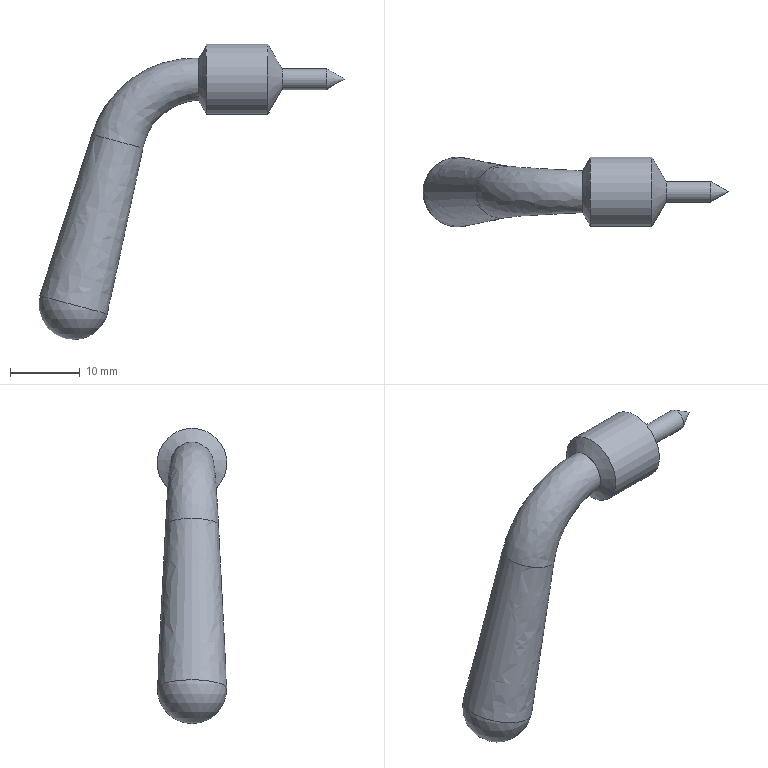Part | NX | features SKETCH 4, DATUM_CSYS 3, DATUM_ON_PATH 2, SKIN 1, SPHERE 1, SWP104 1 | 3 solids | 11 faces | box 43.874 x 10 x 42.344 mm | volume 3412 mm3 | cone 3 | plane 3 | cylinder 2 | spline 2 | sphere 1 | commonest cylinder face diameters 3 x1 10 x1
STEP:
#1=CARTESIAN_POINT('',(18.402,0.,-1.5));
#2=VERTEX_POINT('',#1);
#3=CARTESIAN_POINT('',(18.402,0.,0.));
#4=DIRECTION('',(1.,0.,0.));
#5=DIRECTION('',(0.,0.,-1.));
#6=AXIS2_PLACEMENT_3D('',#3,#4,#5);
#7=CIRCLE('',#6,1.5);
#8=EDGE_CURVE('',#2,#2,#7,.T.);
#9=ORIENTED_EDGE('',*,*,#8,.T.);
#10=EDGE_LOOP('',(#9));
#11=FACE_BOUND('',#10,.T.);
#12=CARTESIAN_POINT('',(21.,0.,0.));
#13=VERTEX_POINT('',#12);
#14=VERTEX_LOOP('',#13);
#15=FACE_BOUND('',#14,.T.);
#16=CARTESIAN_POINT('',(21.,0.,0.));
#17=DIRECTION('',(-1.,0.,0.));
#18=DIRECTION('',(0.,0.,1.));
#19=AXIS2_PLACEMENT_3D('',#16,#17,#18);
#20=CONICAL_SURFACE('',#19,0.,0.5236);
#21=ADVANCED_FACE('',(#11,#15),#20,.T.);
#22=CARTESIAN_POINT('',(12.,0.,-1.5));
#23=VERTEX_POINT('',#22);
#24=CARTESIAN_POINT('',(12.,0.,0.));
#25=DIRECTION('',(1.,0.,0.));
#26=DIRECTION('',(0.,0.,-1.));
#27=AXIS2_PLACEMENT_3D('',#24,#25,#26);
#28=CIRCLE('',#27,1.5);
#29=EDGE_CURVE('',#23,#23,#28,.T.);
#30=ORIENTED_EDGE('',*,*,#29,.T.);
#31=EDGE_LOOP('',(#30));
#32=FACE_BOUND('',#31,.T.);
#33=ORIENTED_EDGE('',*,*,#8,.F.);
#34=EDGE_LOOP('',(#33));
#35=FACE_BOUND('',#34,.T.);
#36=CARTESIAN_POINT('',(0.,0.,0.));
#37=DIRECTION('',(1.,0.,0.));
#38=DIRECTION('',(0.,0.,-1.));
#39=AXIS2_PLACEMENT_3D('',#36,#37,#38);
#40=CYLINDRICAL_SURFACE('',#39,1.5);
#41=ADVANCED_FACE('',(#32,#35),#40,.T.);
#42=CARTESIAN_POINT('',(9.979,0.,-5.));
#43=VERTEX_POINT('',#42);
#44=CARTESIAN_POINT('',(9.979,0.,0.));
#45=DIRECTION('',(1.,0.,0.));
#46=DIRECTION('',(0.,0.,-1.));
#47=AXIS2_PLACEMENT_3D('',#44,#45,#46);
#48=CIRCLE('',#47,5.);
#49=EDGE_CURVE('',#43,#43,#48,.T.);
#50=ORIENTED_EDGE('',*,*,#49,.T.);
#51=EDGE_LOOP('',(#50));
#52=FACE_BOUND('',#51,.T.);
#53=ORIENTED_EDGE('',*,*,#29,.F.);
#54=EDGE_LOOP('',(#53));
#55=FACE_BOUND('',#54,.T.);
#56=CARTESIAN_POINT('',(12.,0.,0.));
#57=DIRECTION('',(-1.,0.,0.));
#58=DIRECTION('',(0.,0.,1.));
#59=AXIS2_PLACEMENT_3D('',#56,#57,#58);
#60=CONICAL_SURFACE('',#59,1.5,1.047);
#61=ADVANCED_FACE('',(#52,#55),#60,.T.);
#62=CARTESIAN_POINT('',(1.155,0.,-5.));
#63=VERTEX_POINT('',#62);
#64=CARTESIAN_POINT('',(1.155,0.,0.));
#65=DIRECTION('',(1.,0.,0.));
#66=DIRECTION('',(0.,0.,-1.));
#67=AXIS2_PLACEMENT_3D('',#64,#65,#66);
#68=CIRCLE('',#67,5.);
#69=EDGE_CURVE('',#63,#63,#68,.T.);
#70=ORIENTED_EDGE('',*,*,#69,.T.);
#71=EDGE_LOOP('',(#70));
#72=FACE_BOUND('',#71,.T.);
#73=ORIENTED_EDGE('',*,*,#49,.F.);
#74=EDGE_LOOP('',(#73));
#75=FACE_BOUND('',#74,.T.);
#76=CARTESIAN_POINT('',(0.,0.,0.));
#77=DIRECTION('',(1.,0.,0.));
#78=DIRECTION('',(0.,0.,-1.));
#79=AXIS2_PLACEMENT_3D('',#76,#77,#78);
#80=CYLINDRICAL_SURFACE('',#79,5.);
#81=ADVANCED_FACE('',(#72,#75),#80,.T.);
#82=CARTESIAN_POINT('',(0.,0.,-3.));
#83=VERTEX_POINT('',#82);
#84=CARTESIAN_POINT('',(0.,0.,0.));
#85=DIRECTION('',(1.,0.,0.));
#86=DIRECTION('',(0.,0.,-1.));
#87=AXIS2_PLACEMENT_3D('',#84,#85,#86);
#88=CIRCLE('',#87,3.);
#89=EDGE_CURVE('',#83,#83,#88,.T.);
#90=ORIENTED_EDGE('',*,*,#89,.T.);
#91=EDGE_LOOP('',(#90));
#92=FACE_BOUND('',#91,.T.);
#93=ORIENTED_EDGE('',*,*,#69,.F.);
#94=EDGE_LOOP('',(#93));
#95=FACE_BOUND('',#94,.T.);
#96=CARTESIAN_POINT('',(1.155,0.,0.));
#97=DIRECTION('',(1.,0.,0.));
#98=DIRECTION('',(0.,0.,-1.));
#99=AXIS2_PLACEMENT_3D('',#96,#97,#98);
#100=CONICAL_SURFACE('',#99,5.,1.047);
#101=ADVANCED_FACE('',(#92,#95),#100,.T.);
#102=ORIENTED_EDGE('',*,*,#89,.F.);
#103=EDGE_LOOP('',(#102));
#104=FACE_BOUND('',#103,.T.);
#105=CARTESIAN_POINT('',(0.,3.,0.));
#106=DIRECTION('',(-1.,0.,0.));
#107=DIRECTION('',(0.,0.,1.));
#108=AXIS2_PLACEMENT_3D('',#105,#106,#107);
#109=PLANE('',#108);
#110=ADVANCED_FACE('',(#104),#109,.T.);
#111=CLOSED_SHELL('',(#21,#41,#61,#81,#101,#110));
#112=MANIFOLD_SOLID_BREP('',#111);
#113=CARTESIAN_POINT('',(-17.874,0.,-37.344));
#114=VERTEX_POINT('',#113);
#115=VERTEX_LOOP('',#114);
#116=FACE_BOUND('',#115,.T.);
#117=CARTESIAN_POINT('',(-17.874,0.,-32.344));
#118=DIRECTION('',(0.,0.,1.));
#119=DIRECTION('',(1.,0.,0.));
#120=AXIS2_PLACEMENT_3D('',#117,#118,#119);
#121=SPHERICAL_SURFACE('',#120,5.);
#122=ADVANCED_FACE('',(#116),#121,.T.);
#123=CLOSED_SHELL('',(#122));
#124=MANIFOLD_SOLID_BREP('',#123);
#125=CARTESIAN_POINT('',(-22.704,0.,-31.05));
#126=VERTEX_POINT('',#125);
#127=CARTESIAN_POINT('',(-22.649,-0.9378,-31.064));
#128=CARTESIAN_POINT('',(-22.729,-0.03039,-31.043));
#129=CARTESIAN_POINT('',(-22.657,0.8728,-31.062));
#130=CARTESIAN_POINT('',(-22.415,1.799,-31.127));
#131=CARTESIAN_POINT('',(-21.975,2.707,-31.245));
#132=CARTESIAN_POINT('',(-21.352,3.522,-31.412));
#133=CARTESIAN_POINT('',(-20.577,4.186,-31.619));
#134=CARTESIAN_POINT('',(-19.707,4.662,-31.853));
#135=CARTESIAN_POINT('',(-18.796,4.938,-32.097));
#136=CARTESIAN_POINT('',(-17.921,5.026,-32.331));
#137=CARTESIAN_POINT('',(-17.048,4.956,-32.565));
#138=CARTESIAN_POINT('',(-16.137,4.701,-32.809));
#139=CARTESIAN_POINT('',(-15.26,4.246,-33.044));
#140=CARTESIAN_POINT('',(-14.472,3.6,-33.255));
#141=CARTESIAN_POINT('',(-13.831,2.798,-33.427));
#142=CARTESIAN_POINT('',(-13.371,1.897,-33.55));
#143=CARTESIAN_POINT('',(-13.104,0.954,-33.622));
#144=CARTESIAN_POINT('',(-13.02,0.04792,-33.645));
#145=CARTESIAN_POINT('',(-13.087,-0.8557,-33.626));
#146=CARTESIAN_POINT('',(-13.334,-1.798,-33.56));
#147=CARTESIAN_POINT('',(-13.773,-2.707,-33.443));
#148=CARTESIAN_POINT('',(-14.397,-3.522,-33.275));
#149=CARTESIAN_POINT('',(-15.172,-4.186,-33.068));
#150=CARTESIAN_POINT('',(-16.042,-4.662,-32.835));
#151=CARTESIAN_POINT('',(-16.953,-4.938,-32.591));
#152=CARTESIAN_POINT('',(-17.828,-5.026,-32.356));
#153=CARTESIAN_POINT('',(-18.701,-4.956,-32.122));
#154=CARTESIAN_POINT('',(-19.612,-4.701,-31.878));
#155=CARTESIAN_POINT('',(-20.489,-4.246,-31.643));
#156=CARTESIAN_POINT('',(-21.276,-3.6,-31.432));
#157=CARTESIAN_POINT('',(-21.918,-2.798,-31.26));
#158=CARTESIAN_POINT('',(-22.378,-1.897,-31.137));
#159=CARTESIAN_POINT('',(-22.649,-0.9378,-31.064));
#160=CARTESIAN_POINT('',(-22.729,-0.03039,-31.043));
#161=CARTESIAN_POINT('',(-22.657,0.8728,-31.062));
#162=B_SPLINE_CURVE_WITH_KNOTS('',3,(#127,#128,#129,#130,#131,#132,#133,#134,#135,#136,#137,#138,#139,#140,#141,#142,#143,#144,#145,#146,#147,#148,#149,#150,#151,#152,#153,#154,#155,#156,#157,#158,#159,#160,#161),.UNSPECIFIED.,.T.,.F.,(1,1,1,1,1,1,1,1,1,1,1,1,1,1,1,1,1,1,1,1,1,1,1,1,1,1,1,1,1,1,1,1,1,1,1,1,1,1,1),(-0.09539,-0.06414,-0.03289,0.,0.02969,0.06086,0.09211,0.1234,0.1546,0.1859,0.2171,0.2484,0.2796,0.3109,0.3421,0.3734,0.4046,0.4359,0.4671,0.4984,0.5296,0.5609,0.5921,0.6234,0.6546,0.6859,0.7171,0.7484,0.7796,0.8109,0.8421,0.8734,0.9046,0.9359,0.9671,1.,1.03,1.061,1.092),.UNSPECIFIED.);
#163=EDGE_CURVE('',#126,#126,#162,.T.);
#164=ORIENTED_EDGE('',*,*,#163,.T.);
#165=EDGE_LOOP('',(#164));
#166=FACE_BOUND('',#165,.T.);
#167=CARTESIAN_POINT('',(-17.874,0.,-32.344));
#168=DIRECTION('',(-0.2588,0.,-0.9659));
#169=DIRECTION('',(0.,1.,0.));
#170=AXIS2_PLACEMENT_3D('',#167,#168,#169);
#171=PLANE('',#170);
#172=ADVANCED_FACE('',(#166),#171,.T.);
#173=CARTESIAN_POINT('',(-15.252,0.,-7.913));
#174=VERTEX_POINT('',#173);
#175=CARTESIAN_POINT('',(-15.252,1.34,-7.913));
#176=CARTESIAN_POINT('',(-15.252,-1.34,-7.913));
#177=CARTESIAN_POINT('',(-14.605,-3.12,-8.087));
#178=CARTESIAN_POINT('',(-12.885,-3.79,-8.547));
#179=CARTESIAN_POINT('',(-10.297,-3.79,-9.241));
#180=CARTESIAN_POINT('',(-8.577,-3.12,-9.702));
#181=CARTESIAN_POINT('',(-7.93,-1.34,-9.875));
#182=CARTESIAN_POINT('',(-7.93,1.34,-9.875));
#183=CARTESIAN_POINT('',(-8.577,3.12,-9.702));
#184=CARTESIAN_POINT('',(-10.297,3.79,-9.241));
#185=CARTESIAN_POINT('',(-12.885,3.79,-8.547));
#186=CARTESIAN_POINT('',(-14.605,3.12,-8.087));
#187=CARTESIAN_POINT('',(-15.252,1.34,-7.913));
#188=CARTESIAN_POINT('',(-15.252,-1.34,-7.913));
#189=(BOUNDED_CURVE()B_SPLINE_CURVE(4,(#175,#176,#177,#178,#179,#180,#181,#182,#183,#184,#185,#186,#187,#188),.UNSPECIFIED.,.T.,.F.)B_SPLINE_CURVE_WITH_KNOTS((2,3,3,3,3,3,2),(-0.25,0.,0.25,0.5,0.75,1.,1.25),.UNSPECIFIED.)CURVE()GEOMETRIC_REPRESENTATION_ITEM()RATIONAL_B_SPLINE_CURVE((0.5858,0.5858,0.5523,0.5858,0.5858,0.5523,0.5858,0.5858,0.5523,0.5858,0.5858,0.5523,0.5858,0.5858))REPRESENTATION_ITEM(''));
#190=EDGE_CURVE('',#174,#174,#189,.F.);
#191=ORIENTED_EDGE('',*,*,#190,.T.);
#192=EDGE_LOOP('',(#191));
#193=FACE_BOUND('',#192,.T.);
#194=ORIENTED_EDGE('',*,*,#163,.F.);
#195=EDGE_LOOP('',(#194));
#196=FACE_BOUND('',#195,.T.);
#197=CARTESIAN_POINT('',(-15.252,1.34,-7.913));
#198=CARTESIAN_POINT('',(-18.978,1.554,-19.481));
#199=CARTESIAN_POINT('',(-22.704,1.768,-31.05));
#200=CARTESIAN_POINT('',(-15.252,-1.34,-7.913));
#201=CARTESIAN_POINT('',(-18.978,-1.554,-19.481));
#202=CARTESIAN_POINT('',(-22.704,-1.768,-31.05));
#203=CARTESIAN_POINT('',(-14.605,-3.12,-8.087));
#204=CARTESIAN_POINT('',(-18.228,-3.618,-19.682));
#205=CARTESIAN_POINT('',(-21.85,-4.116,-31.278));
#206=CARTESIAN_POINT('',(-12.885,-3.79,-8.547));
#207=CARTESIAN_POINT('',(-16.234,-4.395,-20.217));
#208=CARTESIAN_POINT('',(-19.582,-5.,-31.886));
#209=CARTESIAN_POINT('',(-10.297,-3.79,-9.241));
#210=CARTESIAN_POINT('',(-13.232,-4.395,-21.021));
#211=CARTESIAN_POINT('',(-16.167,-5.,-32.801));
#212=CARTESIAN_POINT('',(-8.577,-3.12,-9.702));
#213=CARTESIAN_POINT('',(-11.238,-3.618,-21.555));
#214=CARTESIAN_POINT('',(-13.899,-4.116,-33.409));
#215=CARTESIAN_POINT('',(-7.93,-1.34,-9.875));
#216=CARTESIAN_POINT('',(-10.488,-1.554,-21.756));
#217=CARTESIAN_POINT('',(-13.045,-1.768,-33.638));
#218=CARTESIAN_POINT('',(-7.93,1.34,-9.875));
#219=CARTESIAN_POINT('',(-10.488,1.554,-21.756));
#220=CARTESIAN_POINT('',(-13.045,1.768,-33.638));
#221=CARTESIAN_POINT('',(-8.577,3.12,-9.702));
#222=CARTESIAN_POINT('',(-11.238,3.618,-21.555));
#223=CARTESIAN_POINT('',(-13.899,4.116,-33.409));
#224=CARTESIAN_POINT('',(-10.297,3.79,-9.241));
#225=CARTESIAN_POINT('',(-13.232,4.395,-21.021));
#226=CARTESIAN_POINT('',(-16.167,5.,-32.801));
#227=CARTESIAN_POINT('',(-12.885,3.79,-8.547));
#228=CARTESIAN_POINT('',(-16.234,4.395,-20.217));
#229=CARTESIAN_POINT('',(-19.582,5.,-31.886));
#230=CARTESIAN_POINT('',(-14.605,3.12,-8.087));
#231=CARTESIAN_POINT('',(-18.228,3.618,-19.682));
#232=CARTESIAN_POINT('',(-21.85,4.116,-31.278));
#233=CARTESIAN_POINT('',(-15.252,1.34,-7.913));
#234=CARTESIAN_POINT('',(-18.978,1.554,-19.481));
#235=CARTESIAN_POINT('',(-22.704,1.768,-31.05));
#236=CARTESIAN_POINT('',(-15.252,-1.34,-7.913));
#237=CARTESIAN_POINT('',(-18.978,-1.554,-19.481));
#238=CARTESIAN_POINT('',(-22.704,-1.768,-31.05));
#239=(BOUNDED_SURFACE()B_SPLINE_SURFACE(4,2,((#197,#198,#199),(#200,#201,#202),(#203,#204,#205),(#206,#207,#208),(#209,#210,#211),(#212,#213,#214),(#215,#216,#217),(#218,#219,#220),(#221,#222,#223),(#224,#225,#226),(#227,#228,#229),(#230,#231,#232),(#233,#234,#235),(#236,#237,#238)),.RULED_SURF.,.T.,.F.,.F.)B_SPLINE_SURFACE_WITH_KNOTS((2,3,3,3,3,3,2),(3,3),(-0.25,0.,0.25,0.5,0.75,1.,1.25),(0.,1.),.UNSPECIFIED.)GEOMETRIC_REPRESENTATION_ITEM()RATIONAL_B_SPLINE_SURFACE(((0.5858,0.5858,0.5858),(0.5858,0.5858,0.5858),(0.5523,0.5523,0.5523),(0.5858,0.5858,0.5858),(0.5858,0.5858,0.5858),(0.5523,0.5523,0.5523),(0.5858,0.5858,0.5858),(0.5858,0.5858,0.5858),(0.5523,0.5523,0.5523),(0.5858,0.5858,0.5858),(0.5858,0.5858,0.5858),(0.5523,0.5523,0.5523),(0.5858,0.5858,0.5858),(0.5858,0.5858,0.5858)))REPRESENTATION_ITEM('')SURFACE());
#240=ADVANCED_FACE('',(#193,#196),#239,.F.);
#241=CARTESIAN_POINT('',(0.,0.,3.));
#242=VERTEX_POINT('',#241);
#243=CARTESIAN_POINT('',(0.,0.5627,2.966));
#244=CARTESIAN_POINT('',(0.,0.01824,3.016));
#245=CARTESIAN_POINT('',(0.,-0.5237,2.971));
#246=CARTESIAN_POINT('',(0.,-1.08,2.82));
#247=CARTESIAN_POINT('',(0.,-1.624,2.547));
#248=CARTESIAN_POINT('',(0.,-2.113,2.16));
#249=CARTESIAN_POINT('',(0.,-2.512,1.679));
#250=CARTESIAN_POINT('',(0.,-2.797,1.138));
#251=CARTESIAN_POINT('',(0.,-2.963,0.5724));
#252=CARTESIAN_POINT('',(0.,-3.016,0.02877));
#253=CARTESIAN_POINT('',(0.,-2.974,-0.5134));
#254=CARTESIAN_POINT('',(0.,-2.821,-1.079));
#255=CARTESIAN_POINT('',(0.,-2.547,-1.624));
#256=CARTESIAN_POINT('',(0.,-2.16,-2.113));
#257=CARTESIAN_POINT('',(0.,-1.679,-2.512));
#258=CARTESIAN_POINT('',(0.,-1.138,-2.797));
#259=CARTESIAN_POINT('',(0.,-0.5724,-2.963));
#260=CARTESIAN_POINT('',(0.,-0.02877,-3.016));
#261=CARTESIAN_POINT('',(0.,0.5134,-2.974));
#262=CARTESIAN_POINT('',(0.,1.079,-2.821));
#263=CARTESIAN_POINT('',(0.,1.624,-2.547));
#264=CARTESIAN_POINT('',(0.,2.113,-2.16));
#265=CARTESIAN_POINT('',(0.,2.512,-1.679));
#266=CARTESIAN_POINT('',(0.,2.797,-1.138));
#267=CARTESIAN_POINT('',(0.,2.963,-0.5724));
#268=CARTESIAN_POINT('',(0.,3.016,-0.02877));
#269=CARTESIAN_POINT('',(0.,2.974,0.5134));
#270=CARTESIAN_POINT('',(0.,2.821,1.079));
#271=CARTESIAN_POINT('',(0.,2.547,1.624));
#272=CARTESIAN_POINT('',(0.,2.16,2.113));
#273=CARTESIAN_POINT('',(0.,1.679,2.512));
#274=CARTESIAN_POINT('',(0.,1.138,2.797));
#275=CARTESIAN_POINT('',(0.,0.5627,2.966));
#276=CARTESIAN_POINT('',(0.,0.01824,3.016));
#277=CARTESIAN_POINT('',(0.,-0.5237,2.971));
#278=B_SPLINE_CURVE_WITH_KNOTS('',3,(#243,#244,#245,#246,#247,#248,#249,#250,#251,#252,#253,#254,#255,#256,#257,#258,#259,#260,#261,#262,#263,#264,#265,#266,#267,#268,#269,#270,#271,#272,#273,#274,#275,#276,#277),.UNSPECIFIED.,.T.,.F.,(1,1,1,1,1,1,1,1,1,1,1,1,1,1,1,1,1,1,1,1,1,1,1,1,1,1,1,1,1,1,1,1,1,1,1,1,1,1,1),(-0.09539,-0.06414,-0.03289,0.,0.02969,0.06086,0.09211,0.1234,0.1546,0.1859,0.2171,0.2484,0.2796,0.3109,0.3421,0.3734,0.4046,0.4359,0.4671,0.4984,0.5296,0.5609,0.5921,0.6234,0.6546,0.6859,0.7171,0.7484,0.7796,0.8109,0.8421,0.8734,0.9046,0.9359,0.9671,1.,1.03,1.061,1.092),.UNSPECIFIED.);
#279=EDGE_CURVE('',#242,#242,#278,.T.);
#280=ORIENTED_EDGE('',*,*,#279,.T.);
#281=EDGE_LOOP('',(#280));
#282=FACE_BOUND('',#281,.T.);
#283=CARTESIAN_POINT('',(0.,0.,0.));
#284=DIRECTION('',(-1.,0.,0.));
#285=DIRECTION('',(0.,1.,0.));
#286=AXIS2_PLACEMENT_3D('',#283,#284,#285);
#287=PLANE('',#286);
#288=ADVANCED_FACE('',(#282),#287,.F.);
#289=ORIENTED_EDGE('',*,*,#279,.F.);
#290=EDGE_LOOP('',(#289));
#291=FACE_BOUND('',#290,.T.);
#292=ORIENTED_EDGE('',*,*,#190,.F.);
#293=EDGE_LOOP('',(#292));
#294=FACE_BOUND('',#293,.T.);
#295=CARTESIAN_POINT('',(0.,1.061,3.));
#296=CARTESIAN_POINT('',(-2.423,1.095,3.096));
#297=CARTESIAN_POINT('',(-7.251,1.164,1.713));
#298=CARTESIAN_POINT('',(-11.52,1.236,-1.307));
#299=CARTESIAN_POINT('',(-14.507,1.306,-5.505));
#300=CARTESIAN_POINT('',(-15.252,1.34,-7.913));
#301=CARTESIAN_POINT('',(0.,-1.061,3.));
#302=CARTESIAN_POINT('',(-2.423,-1.095,3.096));
#303=CARTESIAN_POINT('',(-7.251,-1.164,1.713));
#304=CARTESIAN_POINT('',(-11.52,-1.236,-1.307));
#305=CARTESIAN_POINT('',(-14.507,-1.306,-5.505));
#306=CARTESIAN_POINT('',(-15.252,-1.34,-7.913));
#307=CARTESIAN_POINT('',(0.,-2.47,2.47));
#308=CARTESIAN_POINT('',(-2.335,-2.549,2.549));
#309=CARTESIAN_POINT('',(-6.975,-2.711,1.191));
#310=CARTESIAN_POINT('',(-11.061,-2.878,-1.733));
#311=CARTESIAN_POINT('',(-13.904,-3.041,-5.776));
#312=CARTESIAN_POINT('',(-14.605,-3.12,-8.087));
#313=CARTESIAN_POINT('',(0.,-3.,1.061));
#314=CARTESIAN_POINT('',(-2.101,-3.096,1.095));
#315=CARTESIAN_POINT('',(-6.241,-3.293,-0.1958));
#316=CARTESIAN_POINT('',(-9.84,-3.497,-2.867));
#317=CARTESIAN_POINT('',(-12.3,-3.694,-6.494));
#318=CARTESIAN_POINT('',(-12.885,-3.79,-8.547));
#319=CARTESIAN_POINT('',(0.,-3.,-1.061));
#320=CARTESIAN_POINT('',(-1.75,-3.096,-1.095));
#321=CARTESIAN_POINT('',(-5.137,-3.293,-2.284));
#322=CARTESIAN_POINT('',(-8.002,-3.497,-4.573));
#323=CARTESIAN_POINT('',(-9.885,-3.694,-7.574));
#324=CARTESIAN_POINT('',(-10.297,-3.79,-9.241));
#325=CARTESIAN_POINT('',(0.,-2.47,-2.47));
#326=CARTESIAN_POINT('',(-1.517,-2.549,-2.549));
#327=CARTESIAN_POINT('',(-4.404,-2.711,-3.671));
#328=CARTESIAN_POINT('',(-6.781,-2.878,-5.706));
#329=CARTESIAN_POINT('',(-8.282,-3.041,-8.292));
#330=CARTESIAN_POINT('',(-8.577,-3.12,-9.702));
#331=CARTESIAN_POINT('',(0.,-1.061,-3.));
#332=CARTESIAN_POINT('',(-1.429,-1.095,-3.096));
#333=CARTESIAN_POINT('',(-4.128,-1.164,-4.193));
#334=CARTESIAN_POINT('',(-6.322,-1.236,-6.132));
#335=CARTESIAN_POINT('',(-7.678,-1.306,-8.563));
#336=CARTESIAN_POINT('',(-7.93,-1.34,-9.875));
#337=CARTESIAN_POINT('',(0.,1.061,-3.));
#338=CARTESIAN_POINT('',(-1.429,1.095,-3.096));
#339=CARTESIAN_POINT('',(-4.128,1.164,-4.193));
#340=CARTESIAN_POINT('',(-6.322,1.236,-6.132));
#341=CARTESIAN_POINT('',(-7.678,1.306,-8.563));
#342=CARTESIAN_POINT('',(-7.93,1.34,-9.875));
#343=CARTESIAN_POINT('',(0.,2.47,-2.47));
#344=CARTESIAN_POINT('',(-1.517,2.549,-2.549));
#345=CARTESIAN_POINT('',(-4.404,2.711,-3.671));
#346=CARTESIAN_POINT('',(-6.781,2.878,-5.706));
#347=CARTESIAN_POINT('',(-8.282,3.041,-8.292));
#348=CARTESIAN_POINT('',(-8.577,3.12,-9.702));
#349=CARTESIAN_POINT('',(0.,3.,-1.061));
#350=CARTESIAN_POINT('',(-1.75,3.096,-1.095));
#351=CARTESIAN_POINT('',(-5.137,3.293,-2.284));
#352=CARTESIAN_POINT('',(-8.002,3.497,-4.573));
#353=CARTESIAN_POINT('',(-9.885,3.694,-7.574));
#354=CARTESIAN_POINT('',(-10.297,3.79,-9.241));
#355=CARTESIAN_POINT('',(0.,3.,1.061));
#356=CARTESIAN_POINT('',(-2.101,3.096,1.095));
#357=CARTESIAN_POINT('',(-6.241,3.293,-0.1958));
#358=CARTESIAN_POINT('',(-9.84,3.497,-2.867));
#359=CARTESIAN_POINT('',(-12.3,3.694,-6.494));
#360=CARTESIAN_POINT('',(-12.885,3.79,-8.547));
#361=CARTESIAN_POINT('',(0.,2.47,2.47));
#362=CARTESIAN_POINT('',(-2.335,2.549,2.549));
#363=CARTESIAN_POINT('',(-6.975,2.711,1.191));
#364=CARTESIAN_POINT('',(-11.061,2.878,-1.733));
#365=CARTESIAN_POINT('',(-13.904,3.041,-5.776));
#366=CARTESIAN_POINT('',(-14.605,3.12,-8.087));
#367=CARTESIAN_POINT('',(0.,1.061,3.));
#368=CARTESIAN_POINT('',(-2.423,1.095,3.096));
#369=CARTESIAN_POINT('',(-7.251,1.164,1.713));
#370=CARTESIAN_POINT('',(-11.52,1.236,-1.307));
#371=CARTESIAN_POINT('',(-14.507,1.306,-5.505));
#372=CARTESIAN_POINT('',(-15.252,1.34,-7.913));
#373=CARTESIAN_POINT('',(0.,-1.061,3.));
#374=CARTESIAN_POINT('',(-2.423,-1.095,3.096));
#375=CARTESIAN_POINT('',(-7.251,-1.164,1.713));
#376=CARTESIAN_POINT('',(-11.52,-1.236,-1.307));
#377=CARTESIAN_POINT('',(-14.507,-1.306,-5.505));
#378=CARTESIAN_POINT('',(-15.252,-1.34,-7.913));
#379=(BOUNDED_SURFACE()B_SPLINE_SURFACE(4,2,((#295,#296,#297,#298,#299,#300),(#301,#302,#303,#304,#305,#306),(#307,#308,#309,#310,#311,#312),(#313,#314,#315,#316,#317,#318),(#319,#320,#321,#322,#323,#324),(#325,#326,#327,#328,#329,#330),(#331,#332,#333,#334,#335,#336),(#337,#338,#339,#340,#341,#342),(#343,#344,#345,#346,#347,#348),(#349,#350,#351,#352,#353,#354),(#355,#356,#357,#358,#359,#360),(#361,#362,#363,#364,#365,#366),(#367,#368,#369,#370,#371,#372),(#373,#374,#375,#376,#377,#378)),.UNSPECIFIED.,.T.,.F.,.F.)B_SPLINE_SURFACE_WITH_KNOTS((2,3,3,3,3,3,2),(3,1,1,1,3),(-0.25,0.,0.25,0.5,0.75,1.,1.25),(0.,0.25,0.5,0.75,1.),.UNSPECIFIED.)GEOMETRIC_REPRESENTATION_ITEM()RATIONAL_B_SPLINE_SURFACE(((0.5858,0.5555,0.5253,0.5253,0.5555,0.5858),(0.5858,0.5555,0.5253,0.5253,0.5555,0.5858),(0.5523,0.5238,0.4952,0.4952,0.5238,0.5523),(0.5858,0.5555,0.5253,0.5253,0.5555,0.5858),(0.5858,0.5555,0.5253,0.5253,0.5555,0.5858),(0.5523,0.5238,0.4952,0.4952,0.5238,0.5523),(0.5858,0.5555,0.5253,0.5253,0.5555,0.5858),(0.5858,0.5555,0.5253,0.5253,0.5555,0.5858),(0.5523,0.5238,0.4952,0.4952,0.5238,0.5523),(0.5858,0.5555,0.5253,0.5253,0.5555,0.5858),(0.5858,0.5555,0.5253,0.5253,0.5555,0.5858),(0.5523,0.5238,0.4952,0.4952,0.5238,0.5523),(0.5858,0.5555,0.5253,0.5253,0.5555,0.5858),(0.5858,0.5555,0.5253,0.5253,0.5555,0.5858)))REPRESENTATION_ITEM('')SURFACE());
#380=ADVANCED_FACE('',(#291,#294),#379,.F.);
#381=CLOSED_SHELL('',(#172,#240,#288,#380));
#382=MANIFOLD_SOLID_BREP('',#381);
#383=(LENGTH_UNIT()NAMED_UNIT(*)SI_UNIT(.MILLI.,.METRE.));
#384=UNCERTAINTY_MEASURE_WITH_UNIT(LENGTH_MEASURE(0.0508),#383,'','');
#385=(NAMED_UNIT(*)PLANE_ANGLE_UNIT()SI_UNIT($,.RADIAN.));
#386=(NAMED_UNIT(*)SI_UNIT($,.STERADIAN.)SOLID_ANGLE_UNIT());
#387=(GEOMETRIC_REPRESENTATION_CONTEXT(3)GLOBAL_UNCERTAINTY_ASSIGNED_CONTEXT((#384))GLOBAL_UNIT_ASSIGNED_CONTEXT((#383,#385,#386))REPRESENTATION_CONTEXT('',''));
#388=ADVANCED_BREP_SHAPE_REPRESENTATION('',(#112,#124,#382),#387);